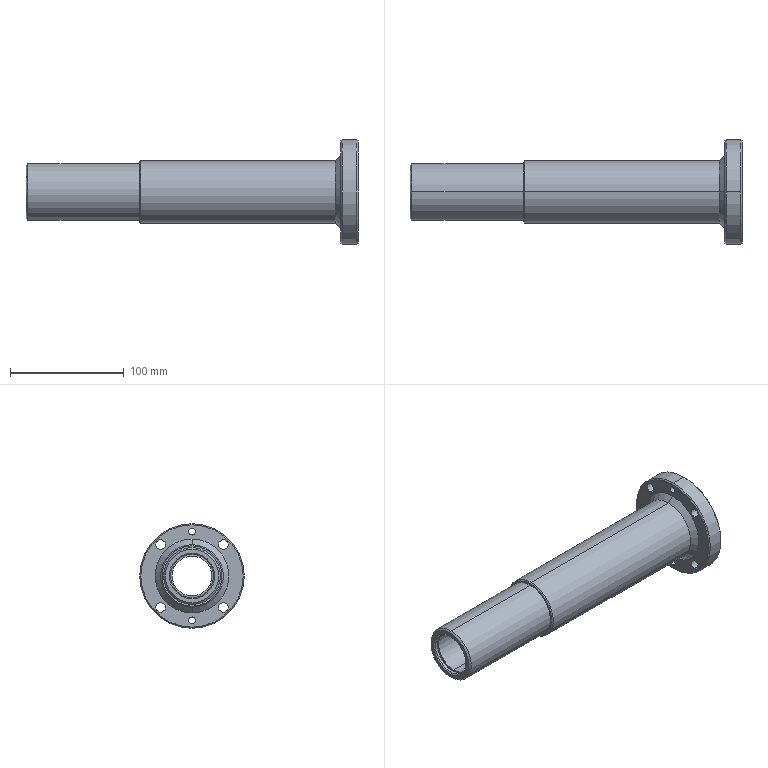Part | STEP file | PN_0061_Default<machined> | 3 solids | 73 faces | box 292 x 92 x 92 mm | volume 411633 mm3 | cylinder 38 | cone 14 | plane 13 | torus 8 | commonest cylinder face diameters 8.5 x8 38 x8 50 x6 6 x4 40.4 x4 55 x4